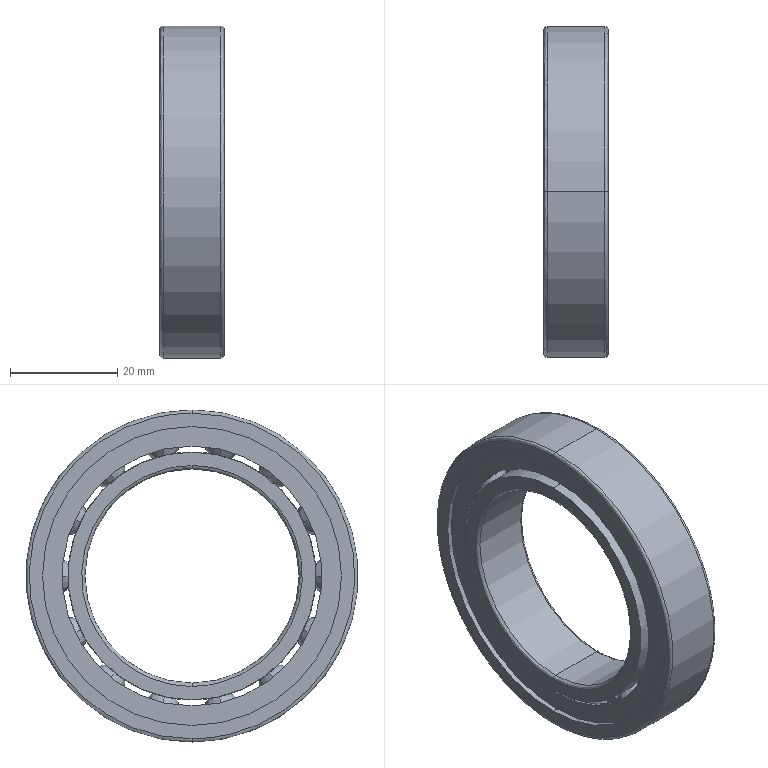Part | STEP file | 1 solid | 225 faces | box 12 x 62 x 62 mm | volume 14109 mm3 | spline 165 | plane 36 | cylinder 24 | commonest cylinder face diameters 55.8 x8 46.3 x4 48.527 x4 40 x2 49.195 x2 52.905 x2